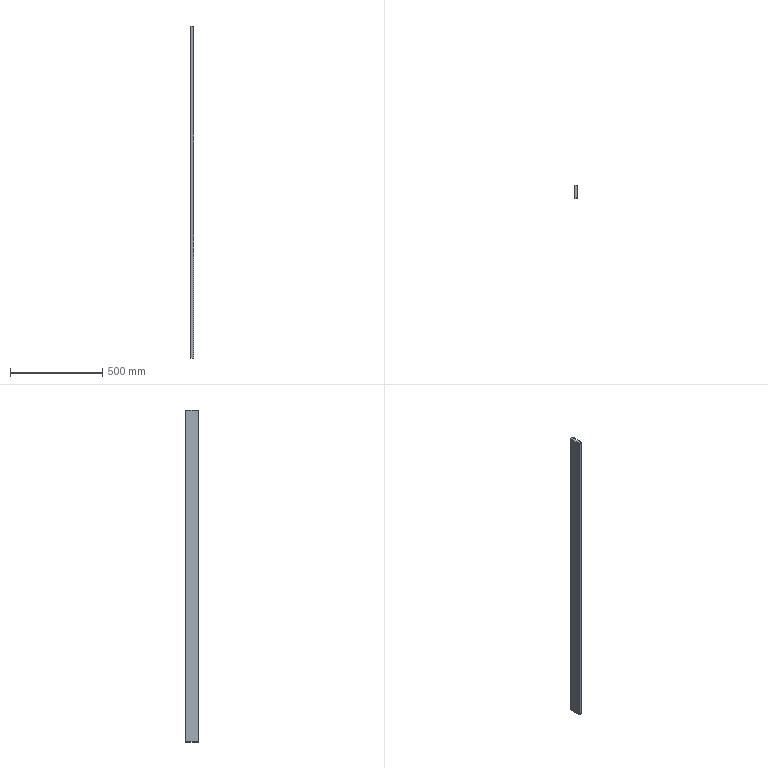Part | SolidWorks | features EdgeFlange 2, FlatPattern 1, ICE 1, LPattern 1, SMBaseFlange 1, SheetMetal 1 | 1 solid | 74 faces | box 20 x 70 x 1800 mm | volume 385797 mm3 | plane 46 | cylinder 28 | commonest cylinder face diameters 6.4 x16 1 x6 4 x6